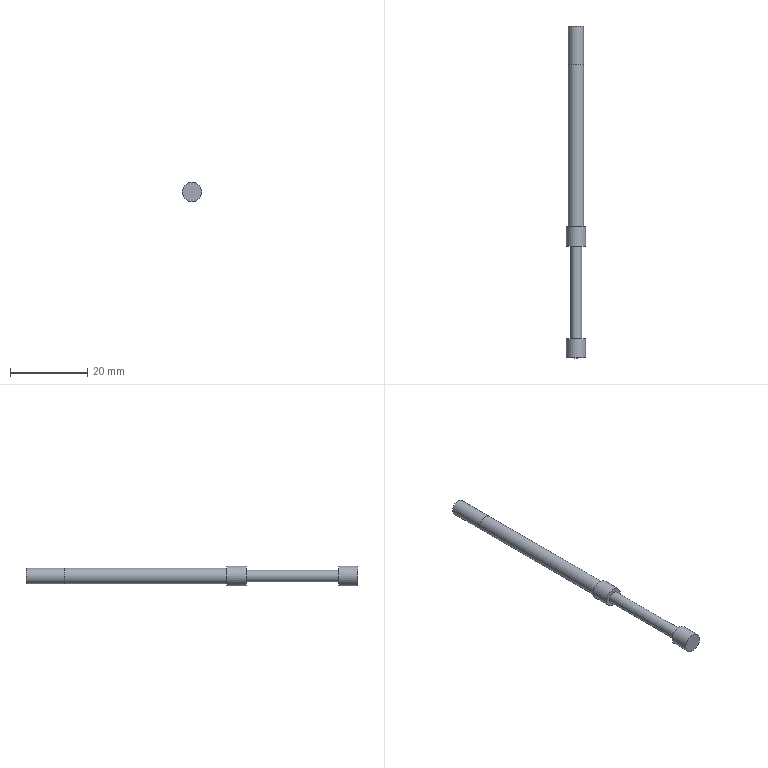Part | STEP file | 2-11.2 | 1 solid | 10 faces | box 5 x 86 x 5 mm | volume 1019 mm3 | cylinder 5 | plane 5 | commonest cylinder face diameters 4 x2 5 x2 3 x1
STEP:
#1=CARTESIAN_POINT('',(0.,0.,0.));
#2=DIRECTION('',(0.,0.,1.));
#3=DIRECTION('',(1.,0.,0.));
#4=AXIS2_PLACEMENT_3D('',#1,#2,#3);
#5=CARTESIAN_POINT('',(1.5,0.,0.));
#6=VERTEX_POINT('',#5);
#7=CARTESIAN_POINT('',(0.,0.,0.));
#8=DIRECTION('',(0.,-1.,0.));
#9=DIRECTION('',(1.,0.,0.));
#10=AXIS2_PLACEMENT_3D('',#7,#8,#9);
#11=CIRCLE('',#10,1.5);
#12=CARTESIAN_POINT('',(0.,0.,0.));
#13=DIRECTION('',(0.,-1.,0.));
#14=DIRECTION('',(1.,0.,0.));
#15=AXIS2_PLACEMENT_3D('',#12,#13,#14);
#16=CYLINDRICAL_SURFACE('',#15,1.5);
#17=CARTESIAN_POINT('',(0.,0.));
#18=DIRECTION('',(1.,0.));
#19=VECTOR('',#18,1.);
#20=LINE('',#17,#19);
#21=(GEOMETRIC_REPRESENTATION_CONTEXT(2)PARAMETRIC_REPRESENTATION_CONTEXT()REPRESENTATION_CONTEXT('',''));
#22=DEFINITIONAL_REPRESENTATION('',(#20),#21);
#23=PCURVE('',#16,#22);
#24=CARTESIAN_POINT('',(-0.6699,0.,0.));
#25=DIRECTION('',(0.,-1.,0.));
#26=DIRECTION('',(1.,0.,0.));
#27=AXIS2_PLACEMENT_3D('',#24,#25,#26);
#28=PLANE('',#27);
#29=CARTESIAN_POINT('',(0.6699,0.));
#30=DIRECTION('',(1.,0.));
#31=AXIS2_PLACEMENT_2D('',#29,#30);
#32=CIRCLE('',#31,1.5);
#33=(GEOMETRIC_REPRESENTATION_CONTEXT(2)PARAMETRIC_REPRESENTATION_CONTEXT()REPRESENTATION_CONTEXT('',''));
#34=DEFINITIONAL_REPRESENTATION('',(#32),#33);
#35=PCURVE('',#28,#34);
#36=SURFACE_CURVE('',#11,(#23,#35),.PCURVE_S1.);
#37=EDGE_CURVE('',#6,#6,#36,.T.);
#38=ORIENTED_EDGE('',*,*,#37,.T.);
#39=CARTESIAN_POINT('',(1.5,-24.,0.));
#40=VERTEX_POINT('',#39);
#41=CARTESIAN_POINT('',(1.5,0.,0.));
#42=DIRECTION('',(0.,-1.,0.));
#43=VECTOR('',#42,1.);
#44=LINE('',#41,#43);
#45=CARTESIAN_POINT('',(6.283,0.));
#46=DIRECTION('',(0.,1.));
#47=VECTOR('',#46,1.);
#48=LINE('',#45,#47);
#49=(GEOMETRIC_REPRESENTATION_CONTEXT(2)PARAMETRIC_REPRESENTATION_CONTEXT()REPRESENTATION_CONTEXT('',''));
#50=DEFINITIONAL_REPRESENTATION('',(#48),#49);
#51=PCURVE('',#16,#50);
#52=CARTESIAN_POINT('',(0.,0.));
#53=DIRECTION('',(0.,1.));
#54=VECTOR('',#53,1.);
#55=LINE('',#52,#54);
#56=(GEOMETRIC_REPRESENTATION_CONTEXT(2)PARAMETRIC_REPRESENTATION_CONTEXT()REPRESENTATION_CONTEXT('',''));
#57=DEFINITIONAL_REPRESENTATION('',(#55),#56);
#58=PCURVE('',#16,#57);
#59=SEAM_CURVE('',#44,(#51,#58),.PCURVE_S1.);
#60=EDGE_CURVE('',#6,#40,#59,.T.);
#61=ORIENTED_EDGE('',*,*,#60,.T.);
#62=CARTESIAN_POINT('',(0.,-24.,0.));
#63=DIRECTION('',(0.,-1.,0.));
#64=DIRECTION('',(1.,0.,0.));
#65=AXIS2_PLACEMENT_3D('',#62,#63,#64);
#66=CIRCLE('',#65,1.5);
#67=CARTESIAN_POINT('',(0.,24.));
#68=DIRECTION('',(1.,0.));
#69=VECTOR('',#68,1.);
#70=LINE('',#67,#69);
#71=(GEOMETRIC_REPRESENTATION_CONTEXT(2)PARAMETRIC_REPRESENTATION_CONTEXT()REPRESENTATION_CONTEXT('',''));
#72=DEFINITIONAL_REPRESENTATION('',(#70),#71);
#73=PCURVE('',#16,#72);
#74=CARTESIAN_POINT('',(-0.6699,-24.,0.));
#75=DIRECTION('',(0.,-1.,0.));
#76=DIRECTION('',(1.,0.,0.));
#77=AXIS2_PLACEMENT_3D('',#74,#75,#76);
#78=PLANE('',#77);
#79=CARTESIAN_POINT('',(0.6699,0.));
#80=DIRECTION('',(1.,0.));
#81=AXIS2_PLACEMENT_2D('',#79,#80);
#82=CIRCLE('',#81,1.5);
#83=(GEOMETRIC_REPRESENTATION_CONTEXT(2)PARAMETRIC_REPRESENTATION_CONTEXT()REPRESENTATION_CONTEXT('',''));
#84=DEFINITIONAL_REPRESENTATION('',(#82),#83);
#85=PCURVE('',#78,#84);
#86=SURFACE_CURVE('',#66,(#73,#85),.PCURVE_S1.);
#87=EDGE_CURVE('',#40,#40,#86,.T.);
#88=ORIENTED_EDGE('',*,*,#87,.F.);
#89=ORIENTED_EDGE('',*,*,#60,.F.);
#90=EDGE_LOOP('',(#38,#61,#88,#89));
#91=FACE_BOUND('',#90,.T.);
#92=ADVANCED_FACE('',(#91),#16,.T.);
#93=CARTESIAN_POINT('',(2.5,-24.,0.));
#94=VERTEX_POINT('',#93);
#95=CARTESIAN_POINT('',(0.,-24.,0.));
#96=DIRECTION('',(0.,-1.,0.));
#97=DIRECTION('',(1.,0.,0.));
#98=AXIS2_PLACEMENT_3D('',#95,#96,#97);
#99=CIRCLE('',#98,2.5);
#100=CARTESIAN_POINT('',(0.6699,0.));
#101=DIRECTION('',(1.,0.));
#102=AXIS2_PLACEMENT_2D('',#100,#101);
#103=CIRCLE('',#102,2.5);
#104=(GEOMETRIC_REPRESENTATION_CONTEXT(2)PARAMETRIC_REPRESENTATION_CONTEXT()REPRESENTATION_CONTEXT('',''));
#105=DEFINITIONAL_REPRESENTATION('',(#103),#104);
#106=PCURVE('',#78,#105);
#107=CARTESIAN_POINT('',(0.,-24.,0.));
#108=DIRECTION('',(0.,-1.,0.));
#109=DIRECTION('',(1.,0.,0.));
#110=AXIS2_PLACEMENT_3D('',#107,#108,#109);
#111=CYLINDRICAL_SURFACE('',#110,2.5);
#112=CARTESIAN_POINT('',(0.,0.));
#113=DIRECTION('',(1.,0.));
#114=VECTOR('',#113,1.);
#115=LINE('',#112,#114);
#116=(GEOMETRIC_REPRESENTATION_CONTEXT(2)PARAMETRIC_REPRESENTATION_CONTEXT()REPRESENTATION_CONTEXT('',''));
#117=DEFINITIONAL_REPRESENTATION('',(#115),#116);
#118=PCURVE('',#111,#117);
#119=SURFACE_CURVE('',#99,(#106,#118),.PCURVE_S1.);
#120=EDGE_CURVE('',#94,#94,#119,.T.);
#121=ORIENTED_EDGE('',*,*,#120,.T.);
#122=EDGE_LOOP('',(#121));
#123=FACE_BOUND('',#122,.F.);
#124=ORIENTED_EDGE('',*,*,#87,.F.);
#125=EDGE_LOOP('',(#124));
#126=FACE_BOUND('',#125,.F.);
#127=ADVANCED_FACE('',(#123,#126),#78,.F.);
#128=ORIENTED_EDGE('',*,*,#120,.T.);
#129=CARTESIAN_POINT('',(2.5,-29.,0.));
#130=VERTEX_POINT('',#129);
#131=CARTESIAN_POINT('',(2.5,-24.,0.));
#132=DIRECTION('',(0.,-1.,0.));
#133=VECTOR('',#132,1.);
#134=LINE('',#131,#133);
#135=CARTESIAN_POINT('',(6.283,0.));
#136=DIRECTION('',(0.,1.));
#137=VECTOR('',#136,1.);
#138=LINE('',#135,#137);
#139=(GEOMETRIC_REPRESENTATION_CONTEXT(2)PARAMETRIC_REPRESENTATION_CONTEXT()REPRESENTATION_CONTEXT('',''));
#140=DEFINITIONAL_REPRESENTATION('',(#138),#139);
#141=PCURVE('',#111,#140);
#142=CARTESIAN_POINT('',(0.,0.));
#143=DIRECTION('',(0.,1.));
#144=VECTOR('',#143,1.);
#145=LINE('',#142,#144);
#146=(GEOMETRIC_REPRESENTATION_CONTEXT(2)PARAMETRIC_REPRESENTATION_CONTEXT()REPRESENTATION_CONTEXT('',''));
#147=DEFINITIONAL_REPRESENTATION('',(#145),#146);
#148=PCURVE('',#111,#147);
#149=SEAM_CURVE('',#134,(#141,#148),.PCURVE_S1.);
#150=EDGE_CURVE('',#94,#130,#149,.T.);
#151=ORIENTED_EDGE('',*,*,#150,.T.);
#152=CARTESIAN_POINT('',(0.,-29.,0.));
#153=DIRECTION('',(0.,-1.,0.));
#154=DIRECTION('',(1.,0.,0.));
#155=AXIS2_PLACEMENT_3D('',#152,#153,#154);
#156=CIRCLE('',#155,2.5);
#157=CARTESIAN_POINT('',(0.,5.));
#158=DIRECTION('',(1.,0.));
#159=VECTOR('',#158,1.);
#160=LINE('',#157,#159);
#161=(GEOMETRIC_REPRESENTATION_CONTEXT(2)PARAMETRIC_REPRESENTATION_CONTEXT()REPRESENTATION_CONTEXT('',''));
#162=DEFINITIONAL_REPRESENTATION('',(#160),#161);
#163=PCURVE('',#111,#162);
#164=CARTESIAN_POINT('',(-0.6699,-29.,0.));
#165=DIRECTION('',(0.,-1.,0.));
#166=DIRECTION('',(1.,0.,0.));
#167=AXIS2_PLACEMENT_3D('',#164,#165,#166);
#168=PLANE('',#167);
#169=CARTESIAN_POINT('',(0.6699,0.));
#170=DIRECTION('',(1.,0.));
#171=AXIS2_PLACEMENT_2D('',#169,#170);
#172=CIRCLE('',#171,2.5);
#173=(GEOMETRIC_REPRESENTATION_CONTEXT(2)PARAMETRIC_REPRESENTATION_CONTEXT()REPRESENTATION_CONTEXT('',''));
#174=DEFINITIONAL_REPRESENTATION('',(#172),#173);
#175=PCURVE('',#168,#174);
#176=SURFACE_CURVE('',#156,(#163,#175),.PCURVE_S1.);
#177=EDGE_CURVE('',#130,#130,#176,.T.);
#178=ORIENTED_EDGE('',*,*,#177,.F.);
#179=ORIENTED_EDGE('',*,*,#150,.F.);
#180=EDGE_LOOP('',(#128,#151,#178,#179));
#181=FACE_BOUND('',#180,.T.);
#182=ADVANCED_FACE('',(#181),#111,.T.);
#183=ORIENTED_EDGE('',*,*,#177,.T.);
#184=EDGE_LOOP('',(#183));
#185=FACE_BOUND('',#184,.T.);
#186=ADVANCED_FACE('',(#185),#168,.T.);
#187=CARTESIAN_POINT('',(2.5,0.,0.));
#188=VERTEX_POINT('',#187);
#189=CARTESIAN_POINT('',(0.,0.,0.));
#190=DIRECTION('',(0.,-1.,0.));
#191=DIRECTION('',(1.,0.,0.));
#192=AXIS2_PLACEMENT_3D('',#189,#190,#191);
#193=CIRCLE('',#192,2.5);
#194=CARTESIAN_POINT('',(0.6699,0.));
#195=DIRECTION('',(1.,0.));
#196=AXIS2_PLACEMENT_2D('',#194,#195);
#197=CIRCLE('',#196,2.5);
#198=(GEOMETRIC_REPRESENTATION_CONTEXT(2)PARAMETRIC_REPRESENTATION_CONTEXT()REPRESENTATION_CONTEXT('',''));
#199=DEFINITIONAL_REPRESENTATION('',(#197),#198);
#200=PCURVE('',#28,#199);
#201=CARTESIAN_POINT('',(0.,0.,0.));
#202=DIRECTION('',(0.,1.,0.));
#203=DIRECTION('',(1.,0.,0.));
#204=AXIS2_PLACEMENT_3D('',#201,#202,#203);
#205=CYLINDRICAL_SURFACE('',#204,2.5);
#206=CARTESIAN_POINT('',(6.283,0.));
#207=DIRECTION('',(-1.,0.));
#208=VECTOR('',#207,1.);
#209=LINE('',#206,#208);
#210=(GEOMETRIC_REPRESENTATION_CONTEXT(2)PARAMETRIC_REPRESENTATION_CONTEXT()REPRESENTATION_CONTEXT('',''));
#211=DEFINITIONAL_REPRESENTATION('',(#209),#210);
#212=PCURVE('',#205,#211);
#213=SURFACE_CURVE('',#193,(#200,#212),.PCURVE_S1.);
#214=EDGE_CURVE('',#188,#188,#213,.T.);
#215=ORIENTED_EDGE('',*,*,#214,.T.);
#216=EDGE_LOOP('',(#215));
#217=FACE_BOUND('',#216,.T.);
#218=ORIENTED_EDGE('',*,*,#37,.F.);
#219=EDGE_LOOP('',(#218));
#220=FACE_BOUND('',#219,.T.);
#221=ADVANCED_FACE('',(#217,#220),#28,.T.);
#222=CARTESIAN_POINT('',(2.5,5.,0.));
#223=VERTEX_POINT('',#222);
#224=CARTESIAN_POINT('',(2.5,0.,0.));
#225=DIRECTION('',(0.,1.,0.));
#226=VECTOR('',#225,1.);
#227=LINE('',#224,#226);
#228=CARTESIAN_POINT('',(6.283,0.));
#229=DIRECTION('',(0.,1.));
#230=VECTOR('',#229,1.);
#231=LINE('',#228,#230);
#232=(GEOMETRIC_REPRESENTATION_CONTEXT(2)PARAMETRIC_REPRESENTATION_CONTEXT()REPRESENTATION_CONTEXT('',''));
#233=DEFINITIONAL_REPRESENTATION('',(#231),#232);
#234=PCURVE('',#205,#233);
#235=CARTESIAN_POINT('',(0.,0.));
#236=DIRECTION('',(0.,1.));
#237=VECTOR('',#236,1.);
#238=LINE('',#235,#237);
#239=(GEOMETRIC_REPRESENTATION_CONTEXT(2)PARAMETRIC_REPRESENTATION_CONTEXT()REPRESENTATION_CONTEXT('',''));
#240=DEFINITIONAL_REPRESENTATION('',(#238),#239);
#241=PCURVE('',#205,#240);
#242=SEAM_CURVE('',#227,(#234,#241),.PCURVE_S1.);
#243=EDGE_CURVE('',#188,#223,#242,.T.);
#244=ORIENTED_EDGE('',*,*,#243,.T.);
#245=CARTESIAN_POINT('',(0.,5.,0.));
#246=DIRECTION('',(0.,-1.,0.));
#247=DIRECTION('',(1.,0.,0.));
#248=AXIS2_PLACEMENT_3D('',#245,#246,#247);
#249=CIRCLE('',#248,2.5);
#250=CARTESIAN_POINT('',(6.283,5.));
#251=DIRECTION('',(-1.,0.));
#252=VECTOR('',#251,1.);
#253=LINE('',#250,#252);
#254=(GEOMETRIC_REPRESENTATION_CONTEXT(2)PARAMETRIC_REPRESENTATION_CONTEXT()REPRESENTATION_CONTEXT('',''));
#255=DEFINITIONAL_REPRESENTATION('',(#253),#254);
#256=PCURVE('',#205,#255);
#257=CARTESIAN_POINT('',(-0.6699,5.,0.));
#258=DIRECTION('',(0.,-1.,0.));
#259=DIRECTION('',(1.,0.,0.));
#260=AXIS2_PLACEMENT_3D('',#257,#258,#259);
#261=PLANE('',#260);
#262=CARTESIAN_POINT('',(0.6699,0.));
#263=DIRECTION('',(1.,0.));
#264=AXIS2_PLACEMENT_2D('',#262,#263);
#265=CIRCLE('',#264,2.5);
#266=(GEOMETRIC_REPRESENTATION_CONTEXT(2)PARAMETRIC_REPRESENTATION_CONTEXT()REPRESENTATION_CONTEXT('',''));
#267=DEFINITIONAL_REPRESENTATION('',(#265),#266);
#268=PCURVE('',#261,#267);
#269=SURFACE_CURVE('',#249,(#256,#268),.PCURVE_S1.);
#270=EDGE_CURVE('',#223,#223,#269,.T.);
#271=ORIENTED_EDGE('',*,*,#270,.T.);
#272=ORIENTED_EDGE('',*,*,#243,.F.);
#273=ORIENTED_EDGE('',*,*,#214,.F.);
#274=EDGE_LOOP('',(#244,#271,#272,#273));
#275=FACE_BOUND('',#274,.T.);
#276=ADVANCED_FACE('',(#275),#205,.T.);
#277=ORIENTED_EDGE('',*,*,#270,.T.);
#278=EDGE_LOOP('',(#277));
#279=FACE_BOUND('',#278,.F.);
#280=CARTESIAN_POINT('',(2.,5.,0.));
#281=VERTEX_POINT('',#280);
#282=CARTESIAN_POINT('',(0.,5.,0.));
#283=DIRECTION('',(0.,-1.,0.));
#284=DIRECTION('',(1.,0.,0.));
#285=AXIS2_PLACEMENT_3D('',#282,#283,#284);
#286=CIRCLE('',#285,2.);
#287=CARTESIAN_POINT('',(0.6699,0.));
#288=DIRECTION('',(1.,0.));
#289=AXIS2_PLACEMENT_2D('',#287,#288);
#290=CIRCLE('',#289,2.);
#291=(GEOMETRIC_REPRESENTATION_CONTEXT(2)PARAMETRIC_REPRESENTATION_CONTEXT()REPRESENTATION_CONTEXT('',''));
#292=DEFINITIONAL_REPRESENTATION('',(#290),#291);
#293=PCURVE('',#261,#292);
#294=CARTESIAN_POINT('',(0.,5.,0.));
#295=DIRECTION('',(0.,1.,0.));
#296=DIRECTION('',(1.,0.,0.));
#297=AXIS2_PLACEMENT_3D('',#294,#295,#296);
#298=CYLINDRICAL_SURFACE('',#297,2.);
#299=CARTESIAN_POINT('',(6.283,0.));
#300=DIRECTION('',(-1.,0.));
#301=VECTOR('',#300,1.);
#302=LINE('',#299,#301);
#303=(GEOMETRIC_REPRESENTATION_CONTEXT(2)PARAMETRIC_REPRESENTATION_CONTEXT()REPRESENTATION_CONTEXT('',''));
#304=DEFINITIONAL_REPRESENTATION('',(#302),#303);
#305=PCURVE('',#298,#304);
#306=SURFACE_CURVE('',#286,(#293,#305),.PCURVE_S1.);
#307=EDGE_CURVE('',#281,#281,#306,.T.);
#308=ORIENTED_EDGE('',*,*,#307,.F.);
#309=EDGE_LOOP('',(#308));
#310=FACE_BOUND('',#309,.F.);
#311=ADVANCED_FACE('',(#279,#310),#261,.F.);
#312=CARTESIAN_POINT('',(2.,57.,0.));
#313=VERTEX_POINT('',#312);
#314=CARTESIAN_POINT('',(0.,57.,0.));
#315=DIRECTION('',(0.,-1.,0.));
#316=DIRECTION('',(1.,0.,0.));
#317=AXIS2_PLACEMENT_3D('',#314,#315,#316);
#318=CIRCLE('',#317,2.);
#319=CARTESIAN_POINT('',(-0.5359,57.,0.));
#320=DIRECTION('',(0.,-1.,0.));
#321=DIRECTION('',(1.,0.,0.));
#322=AXIS2_PLACEMENT_3D('',#319,#320,#321);
#323=PLANE('',#322);
#324=CARTESIAN_POINT('',(0.5359,0.));
#325=DIRECTION('',(1.,0.));
#326=AXIS2_PLACEMENT_2D('',#324,#325);
#327=CIRCLE('',#326,2.);
#328=(GEOMETRIC_REPRESENTATION_CONTEXT(2)PARAMETRIC_REPRESENTATION_CONTEXT()REPRESENTATION_CONTEXT('',''));
#329=DEFINITIONAL_REPRESENTATION('',(#327),#328);
#330=PCURVE('',#323,#329);
#331=CARTESIAN_POINT('',(0.,47.,0.));
#332=DIRECTION('',(0.,1.,0.));
#333=DIRECTION('',(1.,0.,0.));
#334=AXIS2_PLACEMENT_3D('',#331,#332,#333);
#335=CYLINDRICAL_SURFACE('',#334,2.);
#336=CARTESIAN_POINT('',(6.283,10.));
#337=DIRECTION('',(-1.,0.));
#338=VECTOR('',#337,1.);
#339=LINE('',#336,#338);
#340=(GEOMETRIC_REPRESENTATION_CONTEXT(2)PARAMETRIC_REPRESENTATION_CONTEXT()REPRESENTATION_CONTEXT('',''));
#341=DEFINITIONAL_REPRESENTATION('',(#339),#340);
#342=PCURVE('',#335,#341);
#343=SURFACE_CURVE('',#318,(#330,#342),.PCURVE_S1.);
#344=EDGE_CURVE('',#313,#313,#343,.T.);
#345=ORIENTED_EDGE('',*,*,#344,.T.);
#346=EDGE_LOOP('',(#345));
#347=FACE_BOUND('',#346,.F.);
#348=ADVANCED_FACE('',(#347),#323,.F.);
#349=CARTESIAN_POINT('',(2.,47.,0.));
#350=VERTEX_POINT('',#349);
#351=CARTESIAN_POINT('',(2.,5.,0.));
#352=DIRECTION('',(0.,1.,0.));
#353=VECTOR('',#352,1.);
#354=LINE('',#351,#353);
#355=CARTESIAN_POINT('',(6.283,0.));
#356=DIRECTION('',(0.,1.));
#357=VECTOR('',#356,1.);
#358=LINE('',#355,#357);
#359=(GEOMETRIC_REPRESENTATION_CONTEXT(2)PARAMETRIC_REPRESENTATION_CONTEXT()REPRESENTATION_CONTEXT('',''));
#360=DEFINITIONAL_REPRESENTATION('',(#358),#359);
#361=PCURVE('',#298,#360);
#362=CARTESIAN_POINT('',(0.,0.));
#363=DIRECTION('',(0.,1.));
#364=VECTOR('',#363,1.);
#365=LINE('',#362,#364);
#366=(GEOMETRIC_REPRESENTATION_CONTEXT(2)PARAMETRIC_REPRESENTATION_CONTEXT()REPRESENTATION_CONTEXT('',''));
#367=DEFINITIONAL_REPRESENTATION('',(#365),#366);
#368=PCURVE('',#298,#367);
#369=SEAM_CURVE('',#354,(#361,#368),.PCURVE_S1.);
#370=EDGE_CURVE('',#281,#350,#369,.T.);
#371=ORIENTED_EDGE('',*,*,#370,.T.);
#372=CARTESIAN_POINT('',(0.,47.,0.));
#373=DIRECTION('',(0.,-1.,0.));
#374=DIRECTION('',(1.,0.,0.));
#375=AXIS2_PLACEMENT_3D('',#372,#373,#374);
#376=CIRCLE('',#375,2.);
#377=CARTESIAN_POINT('',(6.283,42.));
#378=DIRECTION('',(-1.,0.));
#379=VECTOR('',#378,1.);
#380=LINE('',#377,#379);
#381=(GEOMETRIC_REPRESENTATION_CONTEXT(2)PARAMETRIC_REPRESENTATION_CONTEXT()REPRESENTATION_CONTEXT('',''));
#382=DEFINITIONAL_REPRESENTATION('',(#380),#381);
#383=PCURVE('',#298,#382);
#384=CARTESIAN_POINT('',(6.283,0.));
#385=DIRECTION('',(-1.,0.));
#386=VECTOR('',#385,1.);
#387=LINE('',#384,#386);
#388=(GEOMETRIC_REPRESENTATION_CONTEXT(2)PARAMETRIC_REPRESENTATION_CONTEXT()REPRESENTATION_CONTEXT('',''));
#389=DEFINITIONAL_REPRESENTATION('',(#387),#388);
#390=PCURVE('',#335,#389);
#391=SURFACE_CURVE('',#376,(#383,#390),.PCURVE_S1.);
#392=EDGE_CURVE('',#350,#350,#391,.T.);
#393=ORIENTED_EDGE('',*,*,#392,.T.);
#394=ORIENTED_EDGE('',*,*,#370,.F.);
#395=ORIENTED_EDGE('',*,*,#307,.F.);
#396=EDGE_LOOP('',(#371,#393,#394,#395));
#397=FACE_BOUND('',#396,.T.);
#398=ADVANCED_FACE('',(#397),#298,.T.);
#399=CARTESIAN_POINT('',(2.,47.,0.));
#400=DIRECTION('',(0.,1.,0.));
#401=VECTOR('',#400,1.);
#402=LINE('',#399,#401);
#403=CARTESIAN_POINT('',(0.,0.));
#404=DIRECTION('',(0.,1.));
#405=VECTOR('',#404,1.);
#406=LINE('',#403,#405);
#407=(GEOMETRIC_REPRESENTATION_CONTEXT(2)PARAMETRIC_REPRESENTATION_CONTEXT()REPRESENTATION_CONTEXT('',''));
#408=DEFINITIONAL_REPRESENTATION('',(#406),#407);
#409=PCURVE('',#335,#408);
#410=CARTESIAN_POINT('',(6.283,0.));
#411=DIRECTION('',(0.,1.));
#412=VECTOR('',#411,1.);
#413=LINE('',#410,#412);
#414=(GEOMETRIC_REPRESENTATION_CONTEXT(2)PARAMETRIC_REPRESENTATION_CONTEXT()REPRESENTATION_CONTEXT('',''));
#415=DEFINITIONAL_REPRESENTATION('',(#413),#414);
#416=PCURVE('',#335,#415);
#417=SEAM_CURVE('',#402,(#409,#416),.PCURVE_S1.);
#418=EDGE_CURVE('',#350,#313,#417,.T.);
#419=ORIENTED_EDGE('',*,*,#418,.F.);
#420=ORIENTED_EDGE('',*,*,#392,.F.);
#421=ORIENTED_EDGE('',*,*,#418,.T.);
#422=ORIENTED_EDGE('',*,*,#344,.T.);
#423=EDGE_LOOP('',(#419,#420,#421,#422));
#424=FACE_BOUND('',#423,.T.);
#425=ADVANCED_FACE('',(#424),#335,.T.);
#426=CLOSED_SHELL('',(#92,#127,#182,#186,#221,#276,#311,#348,#398,#425));
#427=MANIFOLD_SOLID_BREP('',#426);
#428=(LENGTH_UNIT()NAMED_UNIT(*)SI_UNIT(.MILLI.,.METRE.));
#429=UNCERTAINTY_MEASURE_WITH_UNIT(LENGTH_MEASURE(0.0000001),#428,'','');
#430=(NAMED_UNIT(*)PLANE_ANGLE_UNIT()SI_UNIT($,.RADIAN.));
#431=(NAMED_UNIT(*)SI_UNIT($,.STERADIAN.)SOLID_ANGLE_UNIT());
#432=(GEOMETRIC_REPRESENTATION_CONTEXT(3)GLOBAL_UNCERTAINTY_ASSIGNED_CONTEXT((#429))GLOBAL_UNIT_ASSIGNED_CONTEXT((#428,#430,#431))REPRESENTATION_CONTEXT('',''));
#433=ADVANCED_BREP_SHAPE_REPRESENTATION('',(#4,#427),#432);